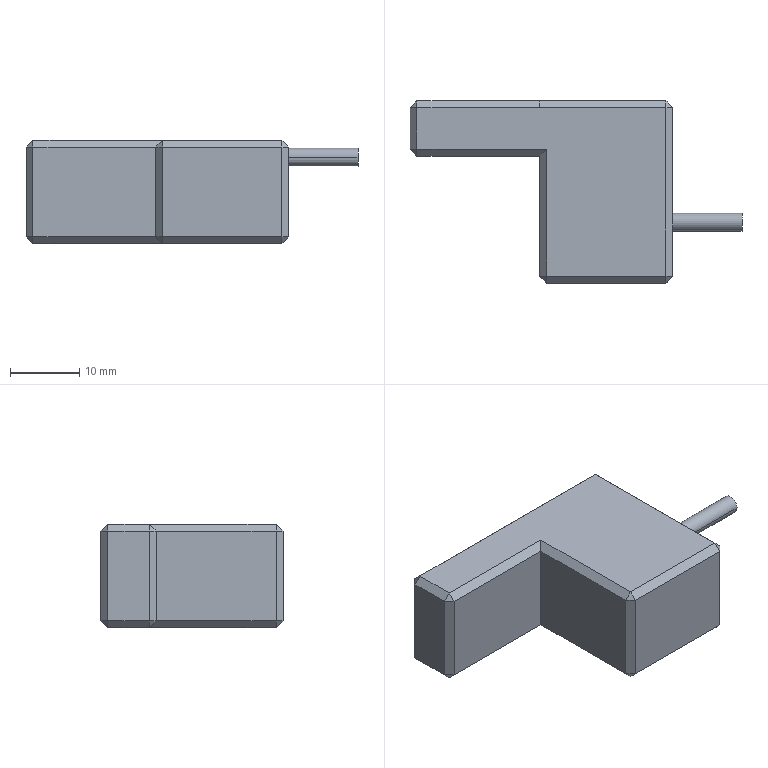Part | SolidWorks | features Chamfer 1, Extrusion 1, ICE 1 | 1 solid | 40 faces | box 48 x 26.348 x 15 mm | volume 9753 mm3 | plane 38 | cylinder 2 | commonest cylinder face diameters 2.6 x2
STEP:
#1=CARTESIAN_POINT('',(-41.415,4.518,5.));
#2=VERTEX_POINT('',#1);
#3=CARTESIAN_POINT('',(-41.415,1.918,5.));
#4=VERTEX_POINT('',#3);
#5=CARTESIAN_POINT('',(-41.415,3.218,5.));
#6=DIRECTION('',(1.,0.,0.));
#7=DIRECTION('',(0.,1.,0.));
#8=AXIS2_PLACEMENT_3D('',#5,#6,#7);
#9=CIRCLE('',#8,1.3);
#10=EDGE_CURVE('',#2,#4,#9,.T.);
#11=ORIENTED_EDGE('',*,*,#10,.F.);
#12=CARTESIAN_POINT('',(-51.415,4.518,5.));
#13=VERTEX_POINT('',#12);
#14=CARTESIAN_POINT('',(-41.415,4.518,5.));
#15=DIRECTION('',(-1.,0.,0.));
#16=VECTOR('',#15,1000.);
#17=LINE('',#14,#16);
#18=EDGE_CURVE('',#2,#13,#17,.T.);
#19=ORIENTED_EDGE('',*,*,#18,.T.);
#20=CARTESIAN_POINT('',(-51.415,1.918,5.));
#21=VERTEX_POINT('',#20);
#22=CARTESIAN_POINT('',(-51.415,3.218,5.));
#23=DIRECTION('',(1.,0.,0.));
#24=DIRECTION('',(0.,-1.,0.));
#25=AXIS2_PLACEMENT_3D('',#22,#23,#24);
#26=CIRCLE('',#25,1.3);
#27=EDGE_CURVE('',#13,#21,#26,.T.);
#28=ORIENTED_EDGE('',*,*,#27,.T.);
#29=CARTESIAN_POINT('',(-41.415,1.918,5.));
#30=DIRECTION('',(-1.,0.,0.));
#31=VECTOR('',#30,1000.);
#32=LINE('',#29,#31);
#33=EDGE_CURVE('',#4,#21,#32,.T.);
#34=ORIENTED_EDGE('',*,*,#33,.F.);
#35=EDGE_LOOP('',(#11,#19,#28,#34));
#36=FACE_OUTER_BOUND('',#35,.T.);
#37=CARTESIAN_POINT('',(-41.415,3.218,5.));
#38=DIRECTION('',(-1.,0.,0.));
#39=DIRECTION('',(0.,-1.,0.));
#40=AXIS2_PLACEMENT_3D('',#37,#38,#39);
#41=CYLINDRICAL_SURFACE('',#40,1.3);
#42=ADVANCED_FACE('',(#36),#41,.T.);
#43=CARTESIAN_POINT('',(-88.415,12.775,6.5));
#44=VERTEX_POINT('',#43);
#45=CARTESIAN_POINT('',(-88.415,12.775,-6.5));
#46=VERTEX_POINT('',#45);
#47=CARTESIAN_POINT('',(-88.415,12.775,7.5));
#48=DIRECTION('',(0.,0.,-1.));
#49=VECTOR('',#48,1000.);
#50=LINE('',#47,#49);
#51=EDGE_CURVE('',#44,#46,#50,.T.);
#52=ORIENTED_EDGE('',*,*,#51,.T.);
#53=CARTESIAN_POINT('',(-70.672,12.775,-6.5));
#54=VERTEX_POINT('',#53);
#55=CARTESIAN_POINT('',(-70.672,12.775,-6.5));
#56=DIRECTION('',(1.,0.,0.));
#57=VECTOR('',#56,1000.);
#58=LINE('',#55,#57);
#59=EDGE_CURVE('',#46,#54,#58,.T.);
#60=ORIENTED_EDGE('',*,*,#59,.T.);
#61=CARTESIAN_POINT('',(-70.672,12.775,6.5));
#62=VERTEX_POINT('',#61);
#63=CARTESIAN_POINT('',(-70.672,12.775,7.5));
#64=DIRECTION('',(0.,0.,-1.));
#65=VECTOR('',#64,1000.);
#66=LINE('',#63,#65);
#67=EDGE_CURVE('',#62,#54,#66,.T.);
#68=ORIENTED_EDGE('',*,*,#67,.F.);
#69=CARTESIAN_POINT('',(-89.415,12.775,6.5));
#70=DIRECTION('',(-1.,0.,0.));
#71=VECTOR('',#70,1000.);
#72=LINE('',#69,#71);
#73=EDGE_CURVE('',#62,#44,#72,.T.);
#74=ORIENTED_EDGE('',*,*,#73,.T.);
#75=EDGE_LOOP('',(#52,#60,#68,#74));
#76=FACE_OUTER_BOUND('',#75,.T.);
#77=CARTESIAN_POINT('',(-89.415,12.775,7.5));
#78=DIRECTION('',(0.,1.,0.));
#79=DIRECTION('',(0.,0.,1.));
#80=AXIS2_PLACEMENT_3D('',#77,#78,#79);
#81=PLANE('',#80);
#82=ADVANCED_FACE('',(#76),#81,.F.);
#83=ORIENTED_EDGE('',*,*,#67,.T.);
#84=CARTESIAN_POINT('',(-70.672,-4.572,-6.5));
#85=VERTEX_POINT('',#84);
#86=CARTESIAN_POINT('',(-70.672,-5.572,-6.5));
#87=DIRECTION('',(0.,-1.,0.));
#88=VECTOR('',#87,1000.);
#89=LINE('',#86,#88);
#90=EDGE_CURVE('',#54,#85,#89,.T.);
#91=ORIENTED_EDGE('',*,*,#90,.T.);
#92=CARTESIAN_POINT('',(-70.672,-4.572,6.5));
#93=VERTEX_POINT('',#92);
#94=CARTESIAN_POINT('',(-70.672,-4.572,7.5));
#95=DIRECTION('',(0.,0.,1.));
#96=VECTOR('',#95,1000.);
#97=LINE('',#94,#96);
#98=EDGE_CURVE('',#85,#93,#97,.T.);
#99=ORIENTED_EDGE('',*,*,#98,.T.);
#100=CARTESIAN_POINT('',(-70.672,5.775,6.5));
#101=DIRECTION('',(0.,1.,0.));
#102=VECTOR('',#101,1000.);
#103=LINE('',#100,#102);
#104=EDGE_CURVE('',#93,#62,#103,.T.);
#105=ORIENTED_EDGE('',*,*,#104,.T.);
#106=EDGE_LOOP('',(#83,#91,#99,#105));
#107=FACE_OUTER_BOUND('',#106,.T.);
#108=CARTESIAN_POINT('',(-70.672,5.775,7.5));
#109=DIRECTION('',(1.,0.,0.));
#110=DIRECTION('',(0.,0.,-1.));
#111=AXIS2_PLACEMENT_3D('',#108,#109,#110);
#112=PLANE('',#111);
#113=ADVANCED_FACE('',(#107),#112,.F.);
#114=CARTESIAN_POINT('',(-69.672,-5.572,6.5));
#115=VERTEX_POINT('',#114);
#116=CARTESIAN_POINT('',(-69.672,-5.572,-6.5));
#117=VERTEX_POINT('',#116);
#118=CARTESIAN_POINT('',(-69.672,-5.572,7.5));
#119=DIRECTION('',(0.,0.,-1.));
#120=VECTOR('',#119,1000.);
#121=LINE('',#118,#120);
#122=EDGE_CURVE('',#115,#117,#121,.T.);
#123=ORIENTED_EDGE('',*,*,#122,.T.);
#124=CARTESIAN_POINT('',(-52.415,-5.572,-6.5));
#125=VERTEX_POINT('',#124);
#126=CARTESIAN_POINT('',(-51.415,-5.572,-6.5));
#127=DIRECTION('',(1.,0.,0.));
#128=VECTOR('',#127,1000.);
#129=LINE('',#126,#128);
#130=EDGE_CURVE('',#117,#125,#129,.T.);
#131=ORIENTED_EDGE('',*,*,#130,.T.);
#132=CARTESIAN_POINT('',(-52.415,-5.572,6.5));
#133=VERTEX_POINT('',#132);
#134=CARTESIAN_POINT('',(-52.415,-5.572,7.5));
#135=DIRECTION('',(0.,0.,1.));
#136=VECTOR('',#135,1000.);
#137=LINE('',#134,#136);
#138=EDGE_CURVE('',#125,#133,#137,.T.);
#139=ORIENTED_EDGE('',*,*,#138,.T.);
#140=CARTESIAN_POINT('',(-70.672,-5.572,6.5));
#141=DIRECTION('',(-1.,0.,0.));
#142=VECTOR('',#141,1000.);
#143=LINE('',#140,#142);
#144=EDGE_CURVE('',#133,#115,#143,.T.);
#145=ORIENTED_EDGE('',*,*,#144,.T.);
#146=EDGE_LOOP('',(#123,#131,#139,#145));
#147=FACE_OUTER_BOUND('',#146,.T.);
#148=CARTESIAN_POINT('',(-70.672,-5.572,7.5));
#149=DIRECTION('',(0.,1.,0.));
#150=DIRECTION('',(0.,0.,1.));
#151=AXIS2_PLACEMENT_3D('',#148,#149,#150);
#152=PLANE('',#151);
#153=ADVANCED_FACE('',(#147),#152,.F.);
#154=CARTESIAN_POINT('',(-51.415,-4.572,-6.5));
#155=VERTEX_POINT('',#154);
#156=CARTESIAN_POINT('',(-51.415,19.775,-6.5));
#157=VERTEX_POINT('',#156);
#158=CARTESIAN_POINT('',(-51.415,20.775,-6.5));
#159=DIRECTION('',(0.,1.,0.));
#160=VECTOR('',#159,1000.);
#161=LINE('',#158,#160);
#162=EDGE_CURVE('',#155,#157,#161,.T.);
#163=ORIENTED_EDGE('',*,*,#162,.T.);
#164=CARTESIAN_POINT('',(-51.415,19.775,6.5));
#165=VERTEX_POINT('',#164);
#166=CARTESIAN_POINT('',(-51.415,19.775,7.5));
#167=DIRECTION('',(0.,0.,1.));
#168=VECTOR('',#167,1000.);
#169=LINE('',#166,#168);
#170=EDGE_CURVE('',#157,#165,#169,.T.);
#171=ORIENTED_EDGE('',*,*,#170,.T.);
#172=CARTESIAN_POINT('',(-51.415,-4.572,6.5));
#173=VERTEX_POINT('',#172);
#174=CARTESIAN_POINT('',(-51.415,5.775,6.5));
#175=DIRECTION('',(0.,-1.,0.));
#176=VECTOR('',#175,1000.);
#177=LINE('',#174,#176);
#178=EDGE_CURVE('',#165,#173,#177,.T.);
#179=ORIENTED_EDGE('',*,*,#178,.T.);
#180=CARTESIAN_POINT('',(-51.415,-4.572,7.5));
#181=DIRECTION('',(0.,0.,-1.));
#182=VECTOR('',#181,1000.);
#183=LINE('',#180,#182);
#184=EDGE_CURVE('',#173,#155,#183,.T.);
#185=ORIENTED_EDGE('',*,*,#184,.T.);
#186=EDGE_LOOP('',(#163,#171,#179,#185));
#187=FACE_OUTER_BOUND('',#186,.T.);
#188=CARTESIAN_POINT('',(-51.415,3.218,5.));
#189=DIRECTION('',(1.,0.,0.));
#190=DIRECTION('',(0.,-1.,0.));
#191=AXIS2_PLACEMENT_3D('',#188,#189,#190);
#192=CIRCLE('',#191,1.3);
#193=EDGE_CURVE('',#21,#13,#192,.T.);
#194=ORIENTED_EDGE('',*,*,#193,.F.);
#195=ORIENTED_EDGE('',*,*,#27,.F.);
#196=EDGE_LOOP('',(#194,#195));
#197=FACE_BOUND('',#196,.T.);
#198=CARTESIAN_POINT('',(-51.415,5.775,7.5));
#199=DIRECTION('',(-1.,0.,0.));
#200=DIRECTION('',(0.,-1.,0.));
#201=AXIS2_PLACEMENT_3D('',#198,#199,#200);
#202=PLANE('',#201);
#203=ADVANCED_FACE('',(#187,#197),#202,.F.);
#204=CARTESIAN_POINT('',(-52.415,20.775,-6.5));
#205=VERTEX_POINT('',#204);
#206=CARTESIAN_POINT('',(-70.672,20.775,-6.5));
#207=VERTEX_POINT('',#206);
#208=CARTESIAN_POINT('',(-89.415,20.775,-6.5));
#209=DIRECTION('',(-1.,0.000000065,0.));
#210=VECTOR('',#209,1000.);
#211=LINE('',#208,#210);
#212=EDGE_CURVE('',#205,#207,#211,.T.);
#213=ORIENTED_EDGE('',*,*,#212,.T.);
#214=CARTESIAN_POINT('',(-88.415,20.775,-6.5));
#215=VERTEX_POINT('',#214);
#216=CARTESIAN_POINT('',(-89.415,20.775,-6.5));
#217=DIRECTION('',(-1.,0.000000065,0.));
#218=VECTOR('',#217,1000.);
#219=LINE('',#216,#218);
#220=EDGE_CURVE('',#207,#215,#219,.T.);
#221=ORIENTED_EDGE('',*,*,#220,.T.);
#222=CARTESIAN_POINT('',(-88.415,20.775,6.5));
#223=VERTEX_POINT('',#222);
#224=CARTESIAN_POINT('',(-88.415,20.775,7.5));
#225=DIRECTION('',(0.,0.,1.));
#226=VECTOR('',#225,1000.);
#227=LINE('',#224,#226);
#228=EDGE_CURVE('',#215,#223,#227,.T.);
#229=ORIENTED_EDGE('',*,*,#228,.T.);
#230=CARTESIAN_POINT('',(-70.672,20.775,6.5));
#231=VERTEX_POINT('',#230);
#232=CARTESIAN_POINT('',(-70.672,20.775,6.5));
#233=DIRECTION('',(1.,-0.000000065,0.));
#234=VECTOR('',#233,1000.);
#235=LINE('',#232,#234);
#236=EDGE_CURVE('',#223,#231,#235,.T.);
#237=ORIENTED_EDGE('',*,*,#236,.T.);
#238=CARTESIAN_POINT('',(-52.415,20.775,6.5));
#239=VERTEX_POINT('',#238);
#240=CARTESIAN_POINT('',(-51.415,20.775,6.5));
#241=DIRECTION('',(1.,-0.000000065,0.));
#242=VECTOR('',#241,1000.);
#243=LINE('',#240,#242);
#244=EDGE_CURVE('',#231,#239,#243,.T.);
#245=ORIENTED_EDGE('',*,*,#244,.T.);
#246=CARTESIAN_POINT('',(-52.415,20.775,-7.5));
#247=DIRECTION('',(0.,0.,-1.));
#248=VECTOR('',#247,1000.);
#249=LINE('',#246,#248);
#250=EDGE_CURVE('',#239,#205,#249,.T.);
#251=ORIENTED_EDGE('',*,*,#250,.T.);
#252=EDGE_LOOP('',(#213,#221,#229,#237,#245,#251));
#253=FACE_OUTER_BOUND('',#252,.T.);
#254=CARTESIAN_POINT('',(-89.415,20.775,7.5));
#255=DIRECTION('',(0.000000065,1.,0.));
#256=DIRECTION('',(-1.,0.000000065,0.));
#257=AXIS2_PLACEMENT_3D('',#254,#255,#256);
#258=PLANE('',#257);
#259=ADVANCED_FACE('',(#253),#258,.T.);
#260=CARTESIAN_POINT('',(-89.415,19.775,6.5));
#261=VERTEX_POINT('',#260);
#262=CARTESIAN_POINT('',(-89.415,19.775,-6.5));
#263=VERTEX_POINT('',#262);
#264=CARTESIAN_POINT('',(-89.415,19.775,-7.5));
#265=DIRECTION('',(0.,0.,-1.));
#266=VECTOR('',#265,1000.);
#267=LINE('',#264,#266);
#268=EDGE_CURVE('',#261,#263,#267,.T.);
#269=ORIENTED_EDGE('',*,*,#268,.T.);
#270=CARTESIAN_POINT('',(-89.415,13.775,-6.5));
#271=VERTEX_POINT('',#270);
#272=CARTESIAN_POINT('',(-89.415,12.775,-6.5));
#273=DIRECTION('',(0.,-1.,0.));
#274=VECTOR('',#273,1000.);
#275=LINE('',#272,#274);
#276=EDGE_CURVE('',#263,#271,#275,.T.);
#277=ORIENTED_EDGE('',*,*,#276,.T.);
#278=CARTESIAN_POINT('',(-89.415,13.775,6.5));
#279=VERTEX_POINT('',#278);
#280=CARTESIAN_POINT('',(-89.415,13.775,7.5));
#281=DIRECTION('',(0.,0.,1.));
#282=VECTOR('',#281,1000.);
#283=LINE('',#280,#282);
#284=EDGE_CURVE('',#271,#279,#283,.T.);
#285=ORIENTED_EDGE('',*,*,#284,.T.);
#286=CARTESIAN_POINT('',(-89.415,15.775,6.5));
#287=DIRECTION('',(0.,1.,0.));
#288=VECTOR('',#287,1000.);
#289=LINE('',#286,#288);
#290=EDGE_CURVE('',#279,#261,#289,.T.);
#291=ORIENTED_EDGE('',*,*,#290,.T.);
#292=EDGE_LOOP('',(#269,#277,#285,#291));
#293=FACE_OUTER_BOUND('',#292,.T.);
#294=CARTESIAN_POINT('',(-89.415,15.775,7.5));
#295=DIRECTION('',(1.,0.,0.));
#296=DIRECTION('',(0.,0.,-1.));
#297=AXIS2_PLACEMENT_3D('',#294,#295,#296);
#298=PLANE('',#297);
#299=ADVANCED_FACE('',(#293),#298,.F.);
#300=CARTESIAN_POINT('',(-52.415,-4.572,7.5));
#301=VERTEX_POINT('',#300);
#302=CARTESIAN_POINT('',(-52.415,19.775,7.5));
#303=VERTEX_POINT('',#302);
#304=CARTESIAN_POINT('',(-52.415,0.,7.5));
#305=DIRECTION('',(0.,1.,0.));
#306=VECTOR('',#305,1000.);
#307=LINE('',#304,#306);
#308=EDGE_CURVE('',#301,#303,#307,.T.);
#309=ORIENTED_EDGE('',*,*,#308,.T.);
#310=CARTESIAN_POINT('',(-70.672,19.775,7.5));
#311=VERTEX_POINT('',#310);
#312=CARTESIAN_POINT('',(-70.672,19.775,7.5));
#313=DIRECTION('',(-1.,0.000000065,0.));
#314=VECTOR('',#313,1000.);
#315=LINE('',#312,#314);
#316=EDGE_CURVE('',#303,#311,#315,.T.);
#317=ORIENTED_EDGE('',*,*,#316,.T.);
#318=CARTESIAN_POINT('',(-88.415,19.775,7.5));
#319=VERTEX_POINT('',#318);
#320=CARTESIAN_POINT('',(-89.415,19.775,7.5));
#321=DIRECTION('',(-1.,0.000000065,0.));
#322=VECTOR('',#321,1000.);
#323=LINE('',#320,#322);
#324=EDGE_CURVE('',#311,#319,#323,.T.);
#325=ORIENTED_EDGE('',*,*,#324,.T.);
#326=CARTESIAN_POINT('',(-88.415,13.775,7.5));
#327=VERTEX_POINT('',#326);
#328=CARTESIAN_POINT('',(-88.415,0.,7.5));
#329=DIRECTION('',(0.,-1.,0.));
#330=VECTOR('',#329,1000.);
#331=LINE('',#328,#330);
#332=EDGE_CURVE('',#319,#327,#331,.T.);
#333=ORIENTED_EDGE('',*,*,#332,.T.);
#334=CARTESIAN_POINT('',(-69.672,13.775,7.5));
#335=VERTEX_POINT('',#334);
#336=CARTESIAN_POINT('',(0.,13.775,7.5));
#337=DIRECTION('',(1.,0.,0.));
#338=VECTOR('',#337,1000.);
#339=LINE('',#336,#338);
#340=EDGE_CURVE('',#327,#335,#339,.T.);
#341=ORIENTED_EDGE('',*,*,#340,.T.);
#342=CARTESIAN_POINT('',(-69.672,-4.572,7.5));
#343=VERTEX_POINT('',#342);
#344=CARTESIAN_POINT('',(-69.672,0.,7.5));
#345=DIRECTION('',(0.,-1.,0.));
#346=VECTOR('',#345,1000.);
#347=LINE('',#344,#346);
#348=EDGE_CURVE('',#335,#343,#347,.T.);
#349=ORIENTED_EDGE('',*,*,#348,.T.);
#350=CARTESIAN_POINT('',(0.,-4.572,7.5));
#351=DIRECTION('',(1.,0.,0.));
#352=VECTOR('',#351,1000.);
#353=LINE('',#350,#352);
#354=EDGE_CURVE('',#343,#301,#353,.T.);
#355=ORIENTED_EDGE('',*,*,#354,.T.);
#356=EDGE_LOOP('',(#309,#317,#325,#333,#341,#349,#355));
#357=FACE_OUTER_BOUND('',#356,.T.);
#358=CARTESIAN_POINT('',(0.,0.,7.5));
#359=DIRECTION('',(0.,0.,-1.));
#360=DIRECTION('',(-1.,0.,0.));
#361=AXIS2_PLACEMENT_3D('',#358,#359,#360);
#362=PLANE('',#361);
#363=ADVANCED_FACE('',(#357),#362,.F.);
#364=CARTESIAN_POINT('',(-52.415,-4.572,-7.5));
#365=VERTEX_POINT('',#364);
#366=CARTESIAN_POINT('',(-69.672,-4.572,-7.5));
#367=VERTEX_POINT('',#366);
#368=CARTESIAN_POINT('',(-70.672,-4.572,-7.5));
#369=DIRECTION('',(-1.,0.,0.));
#370=VECTOR('',#369,1000.);
#371=LINE('',#368,#370);
#372=EDGE_CURVE('',#365,#367,#371,.T.);
#373=ORIENTED_EDGE('',*,*,#372,.T.);
#374=CARTESIAN_POINT('',(-69.672,13.775,-7.5));
#375=VERTEX_POINT('',#374);
#376=CARTESIAN_POINT('',(-69.672,12.775,-7.5));
#377=DIRECTION('',(0.,1.,0.));
#378=VECTOR('',#377,1000.);
#379=LINE('',#376,#378);
#380=EDGE_CURVE('',#367,#375,#379,.T.);
#381=ORIENTED_EDGE('',*,*,#380,.T.);
#382=CARTESIAN_POINT('',(-88.415,13.775,-7.5));
#383=VERTEX_POINT('',#382);
#384=CARTESIAN_POINT('',(-89.415,13.775,-7.5));
#385=DIRECTION('',(-1.,0.,0.));
#386=VECTOR('',#385,1000.);
#387=LINE('',#384,#386);
#388=EDGE_CURVE('',#375,#383,#387,.T.);
#389=ORIENTED_EDGE('',*,*,#388,.T.);
#390=CARTESIAN_POINT('',(-88.415,19.775,-7.5));
#391=VERTEX_POINT('',#390);
#392=CARTESIAN_POINT('',(-88.415,20.775,-7.5));
#393=DIRECTION('',(0.,1.,0.));
#394=VECTOR('',#393,1000.);
#395=LINE('',#392,#394);
#396=EDGE_CURVE('',#383,#391,#395,.T.);
#397=ORIENTED_EDGE('',*,*,#396,.T.);
#398=CARTESIAN_POINT('',(-70.672,19.775,-7.5));
#399=VERTEX_POINT('',#398);
#400=CARTESIAN_POINT('',(0.000001285,19.775,-7.5));
#401=DIRECTION('',(1.,-0.000000065,0.));
#402=VECTOR('',#401,1000.);
#403=LINE('',#400,#402);
#404=EDGE_CURVE('',#391,#399,#403,.T.);
#405=ORIENTED_EDGE('',*,*,#404,.T.);
#406=CARTESIAN_POINT('',(-52.415,19.775,-7.5));
#407=VERTEX_POINT('',#406);
#408=CARTESIAN_POINT('',(0.000001285,19.775,-7.5));
#409=DIRECTION('',(1.,-0.000000065,0.));
#410=VECTOR('',#409,1000.);
#411=LINE('',#408,#410);
#412=EDGE_CURVE('',#399,#407,#411,.T.);
#413=ORIENTED_EDGE('',*,*,#412,.T.);
#414=CARTESIAN_POINT('',(-52.415,-5.572,-7.5));
#415=DIRECTION('',(0.,-1.,0.));
#416=VECTOR('',#415,1000.);
#417=LINE('',#414,#416);
#418=EDGE_CURVE('',#407,#365,#417,.T.);
#419=ORIENTED_EDGE('',*,*,#418,.T.);
#420=EDGE_LOOP('',(#373,#381,#389,#397,#405,#413,#419));
#421=FACE_OUTER_BOUND('',#420,.T.);
#422=CARTESIAN_POINT('',(0.,0.,-7.5));
#423=DIRECTION('',(0.,0.,-1.));
#424=DIRECTION('',(-1.,0.,0.));
#425=AXIS2_PLACEMENT_3D('',#422,#423,#424);
#426=PLANE('',#425);
#427=ADVANCED_FACE('',(#421),#426,.T.);
#428=ORIENTED_EDGE('',*,*,#18,.F.);
#429=CARTESIAN_POINT('',(-41.415,3.218,5.));
#430=DIRECTION('',(1.,0.,0.));
#431=DIRECTION('',(0.,1.,0.));
#432=AXIS2_PLACEMENT_3D('',#429,#430,#431);
#433=CIRCLE('',#432,1.3);
#434=EDGE_CURVE('',#4,#2,#433,.T.);
#435=ORIENTED_EDGE('',*,*,#434,.F.);
#436=ORIENTED_EDGE('',*,*,#33,.T.);
#437=ORIENTED_EDGE('',*,*,#193,.T.);
#438=EDGE_LOOP('',(#428,#435,#436,#437));
#439=FACE_OUTER_BOUND('',#438,.T.);
#440=CARTESIAN_POINT('',(-41.415,3.218,5.));
#441=DIRECTION('',(-1.,0.,0.));
#442=DIRECTION('',(0.,-1.,0.));
#443=AXIS2_PLACEMENT_3D('',#440,#441,#442);
#444=CYLINDRICAL_SURFACE('',#443,1.3);
#445=ADVANCED_FACE('',(#439),#444,.T.);
#446=ORIENTED_EDGE('',*,*,#434,.T.);
#447=ORIENTED_EDGE('',*,*,#10,.T.);
#448=EDGE_LOOP('',(#446,#447));
#449=FACE_OUTER_BOUND('',#448,.T.);
#450=CARTESIAN_POINT('',(-41.415,3.218,5.));
#451=DIRECTION('',(1.,0.,0.));
#452=DIRECTION('',(0.,1.,0.));
#453=AXIS2_PLACEMENT_3D('',#450,#451,#452);
#454=PLANE('',#453);
#455=ADVANCED_FACE('',(#449),#454,.T.);
#456=CARTESIAN_POINT('',(-69.672,-5.072,7.));
#457=DIRECTION('',(0.,0.7071,0.7071));
#458=VECTOR('',#457,1000.);
#459=LINE('',#456,#458);
#460=EDGE_CURVE('',#115,#343,#459,.T.);
#461=ORIENTED_EDGE('',*,*,#460,.F.);
#462=ORIENTED_EDGE('',*,*,#144,.F.);
#463=CARTESIAN_POINT('',(-52.415,-5.072,7.));
#464=DIRECTION('',(0.,-0.7071,-0.7071));
#465=VECTOR('',#464,1000.);
#466=LINE('',#463,#465);
#467=EDGE_CURVE('',#301,#133,#466,.T.);
#468=ORIENTED_EDGE('',*,*,#467,.F.);
#469=ORIENTED_EDGE('',*,*,#354,.F.);
#470=EDGE_LOOP('',(#461,#462,#468,#469));
#471=FACE_OUTER_BOUND('',#470,.T.);
#472=CARTESIAN_POINT('',(0.,-4.572,7.5));
#473=DIRECTION('',(0.,0.7071,-0.7071));
#474=DIRECTION('',(1.,0.,0.));
#475=AXIS2_PLACEMENT_3D('',#472,#473,#474);
#476=PLANE('',#475);
#477=ADVANCED_FACE('',(#471),#476,.F.);
#478=CARTESIAN_POINT('',(-70.672,-4.572,-6.5));
#479=DIRECTION('',(-0.7071,0.7071,0.));
#480=VECTOR('',#479,1000.);
#481=LINE('',#478,#480);
#482=EDGE_CURVE('',#117,#85,#481,.T.);
#483=ORIENTED_EDGE('',*,*,#482,.F.);
#484=ORIENTED_EDGE('',*,*,#122,.F.);
#485=CARTESIAN_POINT('',(-70.672,-4.572,6.5));
#486=DIRECTION('',(0.7071,-0.7071,0.));
#487=VECTOR('',#486,1000.);
#488=LINE('',#485,#487);
#489=EDGE_CURVE('',#93,#115,#488,.T.);
#490=ORIENTED_EDGE('',*,*,#489,.F.);
#491=ORIENTED_EDGE('',*,*,#98,.F.);
#492=EDGE_LOOP('',(#483,#484,#490,#491));
#493=FACE_OUTER_BOUND('',#492,.T.);
#494=CARTESIAN_POINT('',(-69.672,-5.572,7.5));
#495=DIRECTION('',(0.7071,0.7071,0.));
#496=DIRECTION('',(0.,0.,-1.));
#497=AXIS2_PLACEMENT_3D('',#494,#495,#496);
#498=PLANE('',#497);
#499=ADVANCED_FACE('',(#493),#498,.F.);
#500=CARTESIAN_POINT('',(-52.415,-5.572,-6.5));
#501=DIRECTION('',(0.,0.7071,-0.7071));
#502=VECTOR('',#501,1000.);
#503=LINE('',#500,#502);
#504=EDGE_CURVE('',#125,#365,#503,.T.);
#505=ORIENTED_EDGE('',*,*,#504,.F.);
#506=ORIENTED_EDGE('',*,*,#130,.F.);
#507=CARTESIAN_POINT('',(-69.672,-5.072,-7.));
#508=DIRECTION('',(0.,-0.7071,0.7071));
#509=VECTOR('',#508,1000.);
#510=LINE('',#507,#509);
#511=EDGE_CURVE('',#367,#117,#510,.T.);
#512=ORIENTED_EDGE('',*,*,#511,.F.);
#513=ORIENTED_EDGE('',*,*,#372,.F.);
#514=EDGE_LOOP('',(#505,#506,#512,#513));
#515=FACE_OUTER_BOUND('',#514,.T.);
#516=CARTESIAN_POINT('',(-70.672,-5.572,-6.5));
#517=DIRECTION('',(0.,-0.7071,-0.7071));
#518=DIRECTION('',(-1.,0.,0.));
#519=AXIS2_PLACEMENT_3D('',#516,#517,#518);
#520=PLANE('',#519);
#521=ADVANCED_FACE('',(#515),#520,.T.);
#522=CARTESIAN_POINT('',(-51.415,-4.572,6.5));
#523=DIRECTION('',(0.7071,0.7071,0.));
#524=VECTOR('',#523,1000.);
#525=LINE('',#522,#524);
#526=EDGE_CURVE('',#133,#173,#525,.T.);
#527=ORIENTED_EDGE('',*,*,#526,.F.);
#528=ORIENTED_EDGE('',*,*,#138,.F.);
#529=CARTESIAN_POINT('',(-52.415,-5.572,-6.5));
#530=DIRECTION('',(-0.7071,-0.7071,0.));
#531=VECTOR('',#530,1000.);
#532=LINE('',#529,#531);
#533=EDGE_CURVE('',#155,#125,#532,.T.);
#534=ORIENTED_EDGE('',*,*,#533,.F.);
#535=ORIENTED_EDGE('',*,*,#184,.F.);
#536=EDGE_LOOP('',(#527,#528,#534,#535));
#537=FACE_OUTER_BOUND('',#536,.T.);
#538=CARTESIAN_POINT('',(-51.415,-4.572,7.5));
#539=DIRECTION('',(-0.7071,0.7071,0.));
#540=DIRECTION('',(0.,0.,-1.));
#541=AXIS2_PLACEMENT_3D('',#538,#539,#540);
#542=PLANE('',#541);
#543=ADVANCED_FACE('',(#537),#542,.F.);
#544=ORIENTED_EDGE('',*,*,#467,.T.);
#545=ORIENTED_EDGE('',*,*,#526,.T.);
#546=CARTESIAN_POINT('',(-51.415,-4.572,6.5));
#547=DIRECTION('',(0.7071,0.,-0.7071));
#548=VECTOR('',#547,1000.);
#549=LINE('',#546,#548);
#550=EDGE_CURVE('',#301,#173,#549,.T.);
#551=ORIENTED_EDGE('',*,*,#550,.F.);
#552=EDGE_LOOP('',(#544,#545,#551));
#553=FACE_OUTER_BOUND('',#552,.T.);
#554=CARTESIAN_POINT('',(-51.415,-4.572,6.5));
#555=DIRECTION('',(0.5774,-0.5774,0.5774));
#556=DIRECTION('',(0.,-0.7071,-0.7071));
#557=AXIS2_PLACEMENT_3D('',#554,#555,#556);
#558=PLANE('',#557);
#559=ADVANCED_FACE('',(#553),#558,.T.);
#560=ORIENTED_EDGE('',*,*,#489,.T.);
#561=ORIENTED_EDGE('',*,*,#460,.T.);
#562=CARTESIAN_POINT('',(-70.672,-4.572,6.5));
#563=DIRECTION('',(0.7071,0.,0.7071));
#564=VECTOR('',#563,1000.);
#565=LINE('',#562,#564);
#566=EDGE_CURVE('',#93,#343,#565,.T.);
#567=ORIENTED_EDGE('',*,*,#566,.F.);
#568=EDGE_LOOP('',(#560,#561,#567));
#569=FACE_OUTER_BOUND('',#568,.T.);
#570=CARTESIAN_POINT('',(-70.672,-4.572,6.5));
#571=DIRECTION('',(-0.5774,-0.5774,0.5774));
#572=DIRECTION('',(0.7071,0.,0.7071));
#573=AXIS2_PLACEMENT_3D('',#570,#571,#572);
#574=PLANE('',#573);
#575=ADVANCED_FACE('',(#569),#574,.T.);
#576=ORIENTED_EDGE('',*,*,#511,.T.);
#577=ORIENTED_EDGE('',*,*,#482,.T.);
#578=CARTESIAN_POINT('',(-70.672,-4.572,-6.5));
#579=DIRECTION('',(-0.7071,0.,0.7071));
#580=VECTOR('',#579,1000.);
#581=LINE('',#578,#580);
#582=EDGE_CURVE('',#367,#85,#581,.T.);
#583=ORIENTED_EDGE('',*,*,#582,.F.);
#584=EDGE_LOOP('',(#576,#577,#583));
#585=FACE_OUTER_BOUND('',#584,.T.);
#586=CARTESIAN_POINT('',(-70.672,-4.572,-6.5));
#587=DIRECTION('',(-0.5774,-0.5774,-0.5774));
#588=DIRECTION('',(-0.7071,0.,0.7071));
#589=AXIS2_PLACEMENT_3D('',#586,#587,#588);
#590=PLANE('',#589);
#591=ADVANCED_FACE('',(#585),#590,.T.);
#592=ORIENTED_EDGE('',*,*,#533,.T.);
#593=ORIENTED_EDGE('',*,*,#504,.T.);
#594=CARTESIAN_POINT('',(-51.915,-4.572,-7.));
#595=DIRECTION('',(-0.7071,0.,-0.7071));
#596=VECTOR('',#595,1000.);
#597=LINE('',#594,#596);
#598=EDGE_CURVE('',#155,#365,#597,.T.);
#599=ORIENTED_EDGE('',*,*,#598,.F.);
#600=EDGE_LOOP('',(#592,#593,#599));
#601=FACE_OUTER_BOUND('',#600,.T.);
#602=CARTESIAN_POINT('',(-52.415,-5.572,-6.5));
#603=DIRECTION('',(0.5774,-0.5774,-0.5774));
#604=DIRECTION('',(0.,0.7071,-0.7071));
#605=AXIS2_PLACEMENT_3D('',#602,#603,#604);
#606=PLANE('',#605);
#607=ADVANCED_FACE('',(#601),#606,.T.);
#608=ORIENTED_EDGE('',*,*,#550,.T.);
#609=ORIENTED_EDGE('',*,*,#178,.F.);
#610=CARTESIAN_POINT('',(-51.415,19.775,6.5));
#611=DIRECTION('',(0.7071,0.000002631,-0.7071));
#612=VECTOR('',#611,1000.);
#613=LINE('',#610,#612);
#614=EDGE_CURVE('',#303,#165,#613,.T.);
#615=ORIENTED_EDGE('',*,*,#614,.F.);
#616=ORIENTED_EDGE('',*,*,#308,.F.);
#617=EDGE_LOOP('',(#608,#609,#615,#616));
#618=FACE_OUTER_BOUND('',#617,.T.);
#619=CARTESIAN_POINT('',(-52.415,0.,7.5));
#620=DIRECTION('',(-0.7071,0.,-0.7071));
#621=DIRECTION('',(0.,1.,0.));
#622=AXIS2_PLACEMENT_3D('',#619,#620,#621);
#623=PLANE('',#622);
#624=ADVANCED_FACE('',(#618),#623,.F.);
#625=ORIENTED_EDGE('',*,*,#566,.T.);
#626=ORIENTED_EDGE('',*,*,#348,.F.);
#627=CARTESIAN_POINT('',(-74.263,9.183,2.908));
#628=DIRECTION('',(0.5774,0.5774,0.5774));
#629=VECTOR('',#628,1000.);
#630=LINE('',#627,#629);
#631=EDGE_CURVE('',#62,#335,#630,.T.);
#632=ORIENTED_EDGE('',*,*,#631,.F.);
#633=ORIENTED_EDGE('',*,*,#104,.F.);
#634=EDGE_LOOP('',(#625,#626,#632,#633));
#635=FACE_OUTER_BOUND('',#634,.T.);
#636=CARTESIAN_POINT('',(-69.672,0.,7.5));
#637=DIRECTION('',(0.7071,0.,-0.7071));
#638=DIRECTION('',(0.,-1.,0.));
#639=AXIS2_PLACEMENT_3D('',#636,#637,#638);
#640=PLANE('',#639);
#641=ADVANCED_FACE('',(#635),#640,.F.);
#642=ORIENTED_EDGE('',*,*,#582,.T.);
#643=ORIENTED_EDGE('',*,*,#90,.F.);
#644=CARTESIAN_POINT('',(-73.005,10.442,-4.167));
#645=DIRECTION('',(-0.5774,-0.5774,0.5774));
#646=VECTOR('',#645,1000.);
#647=LINE('',#644,#646);
#648=EDGE_CURVE('',#375,#54,#647,.T.);
#649=ORIENTED_EDGE('',*,*,#648,.F.);
#650=ORIENTED_EDGE('',*,*,#380,.F.);
#651=EDGE_LOOP('',(#642,#643,#649,#650));
#652=FACE_OUTER_BOUND('',#651,.T.);
#653=CARTESIAN_POINT('',(-70.672,5.775,-6.5));
#654=DIRECTION('',(-0.7071,0.,-0.7071));
#655=DIRECTION('',(0.,1.,0.));
#656=AXIS2_PLACEMENT_3D('',#653,#654,#655);
#657=PLANE('',#656);
#658=ADVANCED_FACE('',(#652),#657,.T.);
#659=ORIENTED_EDGE('',*,*,#598,.T.);
#660=ORIENTED_EDGE('',*,*,#418,.F.);
#661=CARTESIAN_POINT('',(-51.915,19.775,-7.));
#662=DIRECTION('',(-0.7071,-0.000002631,-0.7071));
#663=VECTOR('',#662,1000.);
#664=LINE('',#661,#663);
#665=EDGE_CURVE('',#157,#407,#664,.T.);
#666=ORIENTED_EDGE('',*,*,#665,.F.);
#667=ORIENTED_EDGE('',*,*,#162,.F.);
#668=EDGE_LOOP('',(#659,#660,#666,#667));
#669=FACE_OUTER_BOUND('',#668,.T.);
#670=CARTESIAN_POINT('',(-51.415,5.775,-6.5));
#671=DIRECTION('',(0.7071,0.,-0.7071));
#672=DIRECTION('',(0.,-1.,0.));
#673=AXIS2_PLACEMENT_3D('',#670,#671,#672);
#674=PLANE('',#673);
#675=ADVANCED_FACE('',(#669),#674,.T.);
#676=CARTESIAN_POINT('',(-51.415,19.775,6.5));
#677=DIRECTION('',(-0.7071,0.7071,0.));
#678=VECTOR('',#677,1000.);
#679=LINE('',#676,#678);
#680=EDGE_CURVE('',#165,#239,#679,.T.);
#681=ORIENTED_EDGE('',*,*,#680,.F.);
#682=ORIENTED_EDGE('',*,*,#170,.F.);
#683=CARTESIAN_POINT('',(-52.415,20.775,-6.5));
#684=DIRECTION('',(0.7071,-0.7071,0.));
#685=VECTOR('',#684,1000.);
#686=LINE('',#683,#685);
#687=EDGE_CURVE('',#205,#157,#686,.T.);
#688=ORIENTED_EDGE('',*,*,#687,.F.);
#689=ORIENTED_EDGE('',*,*,#250,.F.);
#690=EDGE_LOOP('',(#681,#682,#688,#689));
#691=FACE_OUTER_BOUND('',#690,.T.);
#692=CARTESIAN_POINT('',(-52.415,20.775,7.5));
#693=DIRECTION('',(0.7071,0.7071,0.));
#694=DIRECTION('',(0.,0.,1.));
#695=AXIS2_PLACEMENT_3D('',#692,#693,#694);
#696=PLANE('',#695);
#697=ADVANCED_FACE('',(#691),#696,.T.);
#698=ORIENTED_EDGE('',*,*,#614,.T.);
#699=ORIENTED_EDGE('',*,*,#680,.T.);
#700=CARTESIAN_POINT('',(-52.415,20.275,7.));
#701=DIRECTION('',(0.000002631,0.7071,-0.7071));
#702=VECTOR('',#701,1000.);
#703=LINE('',#700,#702);
#704=EDGE_CURVE('',#303,#239,#703,.T.);
#705=ORIENTED_EDGE('',*,*,#704,.F.);
#706=EDGE_LOOP('',(#698,#699,#705));
#707=FACE_OUTER_BOUND('',#706,.T.);
#708=CARTESIAN_POINT('',(-51.415,19.775,6.5));
#709=DIRECTION('',(0.5773,0.5773,0.5774));
#710=DIRECTION('',(0.,-0.7071,0.7071));
#711=AXIS2_PLACEMENT_3D('',#708,#709,#710);
#712=PLANE('',#711);
#713=ADVANCED_FACE('',(#707),#712,.T.);
#714=ORIENTED_EDGE('',*,*,#631,.T.);
#715=ORIENTED_EDGE('',*,*,#340,.F.);
#716=CARTESIAN_POINT('',(-88.415,13.275,7.));
#717=DIRECTION('',(0.,0.7071,0.7071));
#718=VECTOR('',#717,1000.);
#719=LINE('',#716,#718);
#720=EDGE_CURVE('',#44,#327,#719,.T.);
#721=ORIENTED_EDGE('',*,*,#720,.F.);
#722=ORIENTED_EDGE('',*,*,#73,.F.);
#723=EDGE_LOOP('',(#714,#715,#721,#722));
#724=FACE_OUTER_BOUND('',#723,.T.);
#725=CARTESIAN_POINT('',(0.,13.775,7.5));
#726=DIRECTION('',(0.,0.7071,-0.7071));
#727=DIRECTION('',(1.,0.,0.));
#728=AXIS2_PLACEMENT_3D('',#725,#726,#727);
#729=PLANE('',#728);
#730=ADVANCED_FACE('',(#724),#729,.F.);
#731=CARTESIAN_POINT('',(-88.415,12.775,-6.5));
#732=DIRECTION('',(-0.7071,0.7071,0.));
#733=VECTOR('',#732,1000.);
#734=LINE('',#731,#733);
#735=EDGE_CURVE('',#46,#271,#734,.T.);
#736=ORIENTED_EDGE('',*,*,#735,.F.);
#737=ORIENTED_EDGE('',*,*,#51,.F.);
#738=CARTESIAN_POINT('',(-89.415,13.775,6.5));
#739=DIRECTION('',(0.7071,-0.7071,0.));
#740=VECTOR('',#739,1000.);
#741=LINE('',#738,#740);
#742=EDGE_CURVE('',#279,#44,#741,.T.);
#743=ORIENTED_EDGE('',*,*,#742,.F.);
#744=ORIENTED_EDGE('',*,*,#284,.F.);
#745=EDGE_LOOP('',(#736,#737,#743,#744));
#746=FACE_OUTER_BOUND('',#745,.T.);
#747=CARTESIAN_POINT('',(-88.415,12.775,7.5));
#748=DIRECTION('',(0.7071,0.7071,0.));
#749=DIRECTION('',(0.,0.,-1.));
#750=AXIS2_PLACEMENT_3D('',#747,#748,#749);
#751=PLANE('',#750);
#752=ADVANCED_FACE('',(#746),#751,.F.);
#753=ORIENTED_EDGE('',*,*,#648,.T.);
#754=ORIENTED_EDGE('',*,*,#59,.F.);
#755=CARTESIAN_POINT('',(-88.415,12.775,-6.5));
#756=DIRECTION('',(0.,-0.7071,0.7071));
#757=VECTOR('',#756,1000.);
#758=LINE('',#755,#757);
#759=EDGE_CURVE('',#383,#46,#758,.T.);
#760=ORIENTED_EDGE('',*,*,#759,.F.);
#761=ORIENTED_EDGE('',*,*,#388,.F.);
#762=EDGE_LOOP('',(#753,#754,#760,#761));
#763=FACE_OUTER_BOUND('',#762,.T.);
#764=CARTESIAN_POINT('',(-89.415,12.775,-6.5));
#765=DIRECTION('',(0.,-0.7071,-0.7071));
#766=DIRECTION('',(-1.,0.,0.));
#767=AXIS2_PLACEMENT_3D('',#764,#765,#766);
#768=PLANE('',#767);
#769=ADVANCED_FACE('',(#763),#768,.T.);
#770=ORIENTED_EDGE('',*,*,#687,.T.);
#771=ORIENTED_EDGE('',*,*,#665,.T.);
#772=CARTESIAN_POINT('',(-52.415,20.775,-6.5));
#773=DIRECTION('',(-0.000002631,-0.7071,-0.7071));
#774=VECTOR('',#773,1000.);
#775=LINE('',#772,#774);
#776=EDGE_CURVE('',#205,#407,#775,.T.);
#777=ORIENTED_EDGE('',*,*,#776,.F.);
#778=EDGE_LOOP('',(#770,#771,#777));
#779=FACE_OUTER_BOUND('',#778,.T.);
#780=CARTESIAN_POINT('',(-52.415,20.775,-6.5));
#781=DIRECTION('',(0.5773,0.5773,-0.5774));
#782=DIRECTION('',(0.,0.7071,0.7071));
#783=AXIS2_PLACEMENT_3D('',#780,#781,#782);
#784=PLANE('',#783);
#785=ADVANCED_FACE('',(#779),#784,.T.);
#786=ORIENTED_EDGE('',*,*,#704,.T.);
#787=ORIENTED_EDGE('',*,*,#244,.F.);
#788=CARTESIAN_POINT('',(-70.672,19.775,7.5));
#789=DIRECTION('',(0.000000046,0.7071,-0.7071));
#790=VECTOR('',#789,1000.);
#791=LINE('',#788,#790);
#792=EDGE_CURVE('',#311,#231,#791,.T.);
#793=ORIENTED_EDGE('',*,*,#792,.F.);
#794=ORIENTED_EDGE('',*,*,#316,.F.);
#795=EDGE_LOOP('',(#786,#787,#793,#794));
#796=FACE_OUTER_BOUND('',#795,.T.);
#797=CARTESIAN_POINT('',(0.000001285,19.775,7.5));
#798=DIRECTION('',(0.000000046,0.7071,0.7071));
#799=DIRECTION('',(1.,-0.000000065,0.));
#800=AXIS2_PLACEMENT_3D('',#797,#798,#799);
#801=PLANE('',#800);
#802=ADVANCED_FACE('',(#796),#801,.T.);
#803=ORIENTED_EDGE('',*,*,#742,.T.);
#804=ORIENTED_EDGE('',*,*,#720,.T.);
#805=CARTESIAN_POINT('',(-89.415,13.775,6.5));
#806=DIRECTION('',(0.7071,0.,0.7071));
#807=VECTOR('',#806,1000.);
#808=LINE('',#805,#807);
#809=EDGE_CURVE('',#279,#327,#808,.T.);
#810=ORIENTED_EDGE('',*,*,#809,.F.);
#811=EDGE_LOOP('',(#803,#804,#810));
#812=FACE_OUTER_BOUND('',#811,.T.);
#813=CARTESIAN_POINT('',(-89.415,13.775,6.5));
#814=DIRECTION('',(-0.5774,-0.5774,0.5774));
#815=DIRECTION('',(0.7071,0.,0.7071));
#816=AXIS2_PLACEMENT_3D('',#813,#814,#815);
#817=PLANE('',#816);
#818=ADVANCED_FACE('',(#812),#817,.T.);
#819=ORIENTED_EDGE('',*,*,#759,.T.);
#820=ORIENTED_EDGE('',*,*,#735,.T.);
#821=CARTESIAN_POINT('',(-88.915,13.775,-7.));
#822=DIRECTION('',(-0.7071,0.,0.7071));
#823=VECTOR('',#822,1000.);
#824=LINE('',#821,#823);
#825=EDGE_CURVE('',#383,#271,#824,.T.);
#826=ORIENTED_EDGE('',*,*,#825,.F.);
#827=EDGE_LOOP('',(#819,#820,#826));
#828=FACE_OUTER_BOUND('',#827,.T.);
#829=CARTESIAN_POINT('',(-88.415,12.775,-6.5));
#830=DIRECTION('',(-0.5774,-0.5774,-0.5774));
#831=DIRECTION('',(-0.7071,0.,0.7071));
#832=AXIS2_PLACEMENT_3D('',#829,#830,#831);
#833=PLANE('',#832);
#834=ADVANCED_FACE('',(#828),#833,.T.);
#835=ORIENTED_EDGE('',*,*,#776,.T.);
#836=ORIENTED_EDGE('',*,*,#412,.F.);
#837=CARTESIAN_POINT('',(-70.672,20.775,-6.5));
#838=DIRECTION('',(-0.000000046,-0.7071,-0.7071));
#839=VECTOR('',#838,1000.);
#840=LINE('',#837,#839);
#841=EDGE_CURVE('',#207,#399,#840,.T.);
#842=ORIENTED_EDGE('',*,*,#841,.F.);
#843=ORIENTED_EDGE('',*,*,#212,.F.);
#844=EDGE_LOOP('',(#835,#836,#842,#843));
#845=FACE_OUTER_BOUND('',#844,.T.);
#846=CARTESIAN_POINT('',(-89.415,20.775,-6.5));
#847=DIRECTION('',(-0.000000046,-0.7071,0.7071));
#848=DIRECTION('',(-1.,0.000000065,0.));
#849=AXIS2_PLACEMENT_3D('',#846,#847,#848);
#850=PLANE('',#849);
#851=ADVANCED_FACE('',(#845),#850,.F.);
#852=ORIENTED_EDGE('',*,*,#792,.T.);
#853=ORIENTED_EDGE('',*,*,#236,.F.);
#854=CARTESIAN_POINT('',(-88.415,20.775,6.5));
#855=DIRECTION('',(0.,0.7071,-0.7071));
#856=VECTOR('',#855,1000.);
#857=LINE('',#854,#856);
#858=EDGE_CURVE('',#319,#223,#857,.T.);
#859=ORIENTED_EDGE('',*,*,#858,.F.);
#860=ORIENTED_EDGE('',*,*,#324,.F.);
#861=EDGE_LOOP('',(#852,#853,#859,#860));
#862=FACE_OUTER_BOUND('',#861,.T.);
#863=CARTESIAN_POINT('',(-89.415,20.775,6.5));
#864=DIRECTION('',(0.000000046,0.7071,0.7071));
#865=DIRECTION('',(-1.,0.000000065,0.));
#866=AXIS2_PLACEMENT_3D('',#863,#864,#865);
#867=PLANE('',#866);
#868=ADVANCED_FACE('',(#862),#867,.T.);
#869=ORIENTED_EDGE('',*,*,#809,.T.);
#870=ORIENTED_EDGE('',*,*,#332,.F.);
#871=CARTESIAN_POINT('',(-88.915,19.775,7.));
#872=DIRECTION('',(0.7071,-0.000000092,0.7071));
#873=VECTOR('',#872,1000.);
#874=LINE('',#871,#873);
#875=EDGE_CURVE('',#261,#319,#874,.T.);
#876=ORIENTED_EDGE('',*,*,#875,.F.);
#877=ORIENTED_EDGE('',*,*,#290,.F.);
#878=EDGE_LOOP('',(#869,#870,#876,#877));
#879=FACE_OUTER_BOUND('',#878,.T.);
#880=CARTESIAN_POINT('',(-88.415,0.,7.5));
#881=DIRECTION('',(0.7071,0.,-0.7071));
#882=DIRECTION('',(0.,-1.,0.));
#883=AXIS2_PLACEMENT_3D('',#880,#881,#882);
#884=PLANE('',#883);
#885=ADVANCED_FACE('',(#879),#884,.F.);
#886=ORIENTED_EDGE('',*,*,#825,.T.);
#887=ORIENTED_EDGE('',*,*,#276,.F.);
#888=CARTESIAN_POINT('',(-89.415,19.775,-6.5));
#889=DIRECTION('',(-0.7071,0.000000092,0.7071));
#890=VECTOR('',#889,1000.);
#891=LINE('',#888,#890);
#892=EDGE_CURVE('',#391,#263,#891,.T.);
#893=ORIENTED_EDGE('',*,*,#892,.F.);
#894=ORIENTED_EDGE('',*,*,#396,.F.);
#895=EDGE_LOOP('',(#886,#887,#893,#894));
#896=FACE_OUTER_BOUND('',#895,.T.);
#897=CARTESIAN_POINT('',(-89.415,15.775,-6.5));
#898=DIRECTION('',(-0.7071,0.,-0.7071));
#899=DIRECTION('',(0.,1.,0.));
#900=AXIS2_PLACEMENT_3D('',#897,#898,#899);
#901=PLANE('',#900);
#902=ADVANCED_FACE('',(#896),#901,.T.);
#903=ORIENTED_EDGE('',*,*,#841,.T.);
#904=ORIENTED_EDGE('',*,*,#404,.F.);
#905=CARTESIAN_POINT('',(-88.415,20.275,-7.));
#906=DIRECTION('',(0.,-0.7071,-0.7071));
#907=VECTOR('',#906,1000.);
#908=LINE('',#905,#907);
#909=EDGE_CURVE('',#215,#391,#908,.T.);
#910=ORIENTED_EDGE('',*,*,#909,.F.);
#911=ORIENTED_EDGE('',*,*,#220,.F.);
#912=EDGE_LOOP('',(#903,#904,#910,#911));
#913=FACE_OUTER_BOUND('',#912,.T.);
#914=CARTESIAN_POINT('',(0.000001285,19.775,-7.5));
#915=DIRECTION('',(-0.000000046,-0.7071,0.7071));
#916=DIRECTION('',(1.,-0.000000065,0.));
#917=AXIS2_PLACEMENT_3D('',#914,#915,#916);
#918=PLANE('',#917);
#919=ADVANCED_FACE('',(#913),#918,.F.);
#920=ORIENTED_EDGE('',*,*,#875,.T.);
#921=ORIENTED_EDGE('',*,*,#858,.T.);
#922=CARTESIAN_POINT('',(-88.415,20.775,6.5));
#923=DIRECTION('',(0.7071,0.7071,0.));
#924=VECTOR('',#923,1000.);
#925=LINE('',#922,#924);
#926=EDGE_CURVE('',#261,#223,#925,.T.);
#927=ORIENTED_EDGE('',*,*,#926,.F.);
#928=EDGE_LOOP('',(#920,#921,#927));
#929=FACE_OUTER_BOUND('',#928,.T.);
#930=CARTESIAN_POINT('',(-88.415,20.775,6.5));
#931=DIRECTION('',(-0.5774,0.5774,0.5774));
#932=DIRECTION('',(0.,-0.7071,0.7071));
#933=AXIS2_PLACEMENT_3D('',#930,#931,#932);
#934=PLANE('',#933);
#935=ADVANCED_FACE('',(#929),#934,.T.);
#936=ORIENTED_EDGE('',*,*,#909,.T.);
#937=ORIENTED_EDGE('',*,*,#892,.T.);
#938=CARTESIAN_POINT('',(-89.415,19.775,-6.5));
#939=DIRECTION('',(-0.7071,-0.7071,0.));
#940=VECTOR('',#939,1000.);
#941=LINE('',#938,#940);
#942=EDGE_CURVE('',#215,#263,#941,.T.);
#943=ORIENTED_EDGE('',*,*,#942,.F.);
#944=EDGE_LOOP('',(#936,#937,#943));
#945=FACE_OUTER_BOUND('',#944,.T.);
#946=CARTESIAN_POINT('',(-89.415,19.775,-6.5));
#947=DIRECTION('',(-0.5774,0.5774,-0.5774));
#948=DIRECTION('',(0.,0.7071,0.7071));
#949=AXIS2_PLACEMENT_3D('',#946,#947,#948);
#950=PLANE('',#949);
#951=ADVANCED_FACE('',(#945),#950,.T.);
#952=ORIENTED_EDGE('',*,*,#926,.T.);
#953=ORIENTED_EDGE('',*,*,#228,.F.);
#954=ORIENTED_EDGE('',*,*,#942,.T.);
#955=ORIENTED_EDGE('',*,*,#268,.F.);
#956=EDGE_LOOP('',(#952,#953,#954,#955));
#957=FACE_OUTER_BOUND('',#956,.T.);
#958=CARTESIAN_POINT('',(-89.415,19.775,7.5));
#959=DIRECTION('',(-0.7071,0.7071,0.));
#960=DIRECTION('',(0.,0.,1.));
#961=AXIS2_PLACEMENT_3D('',#958,#959,#960);
#962=PLANE('',#961);
#963=ADVANCED_FACE('',(#957),#962,.T.);
#964=CLOSED_SHELL('',(#42,#82,#113,#153,#203,#259,#299,#363,#427,#445,#455,#477,#499,#521,#543,#559,#575,#591,#607,#624,#641,#658,#675,#697,#713,#730,#752,#769,#785,#802,#818,#834,#851,#868,#885,#902,#919,#935,#951,#963));
#965=MANIFOLD_SOLID_BREP('',#964);
#966=CARTESIAN_POINT('',(0.,0.,0.));
#967=DIRECTION('',(0.,0.,1.));
#968=DIRECTION('',(1.,0.,0.));
#969=AXIS2_PLACEMENT_3D('',#966,#967,#968);
#970=(LENGTH_UNIT()NAMED_UNIT(*)SI_UNIT(.MILLI.,.METRE.));
#971=UNCERTAINTY_MEASURE_WITH_UNIT(LENGTH_MEASURE(0.00001),#970,'','');
#972=(NAMED_UNIT(*)PLANE_ANGLE_UNIT()SI_UNIT($,.RADIAN.));
#973=(NAMED_UNIT(*)SI_UNIT($,.STERADIAN.)SOLID_ANGLE_UNIT());
#974=(GEOMETRIC_REPRESENTATION_CONTEXT(3)GLOBAL_UNCERTAINTY_ASSIGNED_CONTEXT((#971))GLOBAL_UNIT_ASSIGNED_CONTEXT((#970,#972,#973))REPRESENTATION_CONTEXT('',''));
#975=ADVANCED_BREP_SHAPE_REPRESENTATION('',(#965,#969),#974);